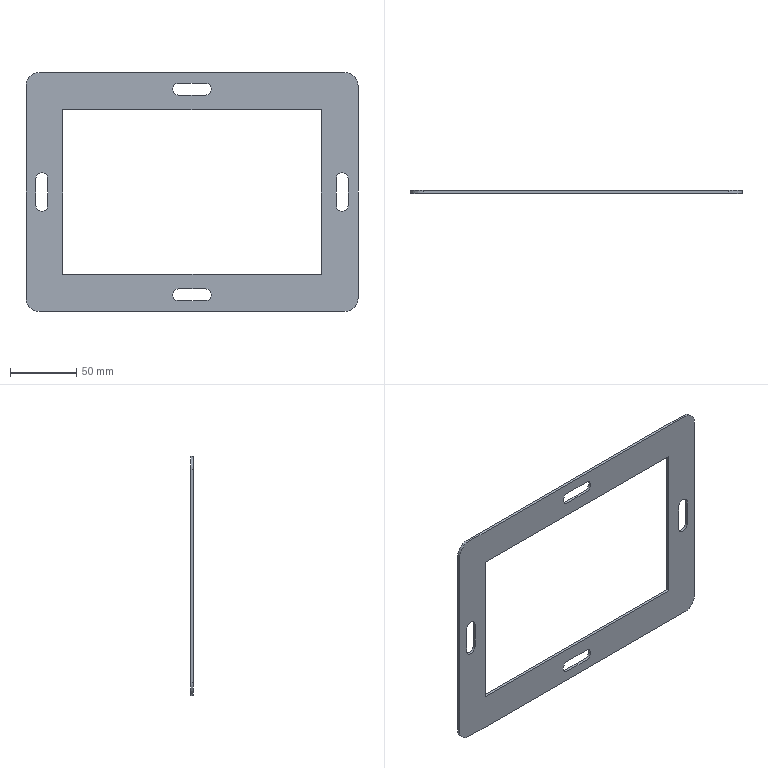Part | STEP file | JBJ-P-1003-01 | 1 solid | 30 faces | box 250 x 2 x 180 mm | volume 39519 mm3 | plane 18 | cylinder 12 | commonest cylinder face diameters 9 x8 20 x4
STEP:
#1=CARTESIAN_POINT('',(125.,2.,80.));
#2=VERTEX_POINT('',#1);
#3=CARTESIAN_POINT('',(125.,2.,-80.));
#4=VERTEX_POINT('',#3);
#5=CARTESIAN_POINT('',(125.,2.,-90.));
#6=DIRECTION('',(0.,0.,-1.));
#7=VECTOR('',#6,1000.);
#8=LINE('',#5,#7);
#9=EDGE_CURVE('',#2,#4,#8,.T.);
#10=ORIENTED_EDGE('',*,*,#9,.F.);
#11=CARTESIAN_POINT('',(125.,0.,80.));
#12=VERTEX_POINT('',#11);
#13=CARTESIAN_POINT('',(125.,2.,80.));
#14=DIRECTION('',(0.,-1.,0.));
#15=VECTOR('',#14,1000.);
#16=LINE('',#13,#15);
#17=EDGE_CURVE('',#2,#12,#16,.T.);
#18=ORIENTED_EDGE('',*,*,#17,.T.);
#19=CARTESIAN_POINT('',(125.,0.,-80.));
#20=VERTEX_POINT('',#19);
#21=CARTESIAN_POINT('',(125.,0.,-90.));
#22=DIRECTION('',(0.,0.,-1.));
#23=VECTOR('',#22,1000.);
#24=LINE('',#21,#23);
#25=EDGE_CURVE('',#12,#20,#24,.T.);
#26=ORIENTED_EDGE('',*,*,#25,.T.);
#27=CARTESIAN_POINT('',(125.,2.,-80.));
#28=DIRECTION('',(0.,1.,0.));
#29=VECTOR('',#28,1000.);
#30=LINE('',#27,#29);
#31=EDGE_CURVE('',#20,#4,#30,.T.);
#32=ORIENTED_EDGE('',*,*,#31,.T.);
#33=EDGE_LOOP('',(#10,#18,#26,#32));
#34=FACE_OUTER_BOUND('',#33,.T.);
#35=CARTESIAN_POINT('',(125.,2.,-90.));
#36=DIRECTION('',(-1.,0.,0.));
#37=DIRECTION('',(0.,0.,1.));
#38=AXIS2_PLACEMENT_3D('',#35,#36,#37);
#39=PLANE('',#38);
#40=ADVANCED_FACE('',(#34),#39,.F.);
#41=CARTESIAN_POINT('',(115.,2.,-90.));
#42=VERTEX_POINT('',#41);
#43=CARTESIAN_POINT('',(-115.,2.,-90.));
#44=VERTEX_POINT('',#43);
#45=CARTESIAN_POINT('',(-125.,2.,-90.));
#46=DIRECTION('',(-1.,0.,0.));
#47=VECTOR('',#46,1000.);
#48=LINE('',#45,#47);
#49=EDGE_CURVE('',#42,#44,#48,.T.);
#50=ORIENTED_EDGE('',*,*,#49,.F.);
#51=CARTESIAN_POINT('',(115.,0.,-90.));
#52=VERTEX_POINT('',#51);
#53=CARTESIAN_POINT('',(115.,2.,-90.));
#54=DIRECTION('',(0.,-1.,0.));
#55=VECTOR('',#54,1000.);
#56=LINE('',#53,#55);
#57=EDGE_CURVE('',#42,#52,#56,.T.);
#58=ORIENTED_EDGE('',*,*,#57,.T.);
#59=CARTESIAN_POINT('',(-115.,0.,-90.));
#60=VERTEX_POINT('',#59);
#61=CARTESIAN_POINT('',(-125.,0.,-90.));
#62=DIRECTION('',(-1.,0.,0.));
#63=VECTOR('',#62,1000.);
#64=LINE('',#61,#63);
#65=EDGE_CURVE('',#52,#60,#64,.T.);
#66=ORIENTED_EDGE('',*,*,#65,.T.);
#67=CARTESIAN_POINT('',(-115.,2.,-90.));
#68=DIRECTION('',(0.,1.,0.));
#69=VECTOR('',#68,1000.);
#70=LINE('',#67,#69);
#71=EDGE_CURVE('',#60,#44,#70,.T.);
#72=ORIENTED_EDGE('',*,*,#71,.T.);
#73=EDGE_LOOP('',(#50,#58,#66,#72));
#74=FACE_OUTER_BOUND('',#73,.T.);
#75=CARTESIAN_POINT('',(-125.,2.,-90.));
#76=DIRECTION('',(0.,0.,1.));
#77=DIRECTION('',(1.,0.,0.));
#78=AXIS2_PLACEMENT_3D('',#75,#76,#77);
#79=PLANE('',#78);
#80=ADVANCED_FACE('',(#74),#79,.F.);
#81=CARTESIAN_POINT('',(-125.,0.,-80.));
#82=VERTEX_POINT('',#81);
#83=CARTESIAN_POINT('',(-125.,0.,80.));
#84=VERTEX_POINT('',#83);
#85=CARTESIAN_POINT('',(-125.,0.,-90.));
#86=DIRECTION('',(0.,0.,1.));
#87=VECTOR('',#86,1000.);
#88=LINE('',#85,#87);
#89=EDGE_CURVE('',#82,#84,#88,.T.);
#90=ORIENTED_EDGE('',*,*,#89,.T.);
#91=CARTESIAN_POINT('',(-125.,2.,80.));
#92=VERTEX_POINT('',#91);
#93=CARTESIAN_POINT('',(-125.,2.,80.));
#94=DIRECTION('',(0.,1.,0.));
#95=VECTOR('',#94,1000.);
#96=LINE('',#93,#95);
#97=EDGE_CURVE('',#84,#92,#96,.T.);
#98=ORIENTED_EDGE('',*,*,#97,.T.);
#99=CARTESIAN_POINT('',(-125.,2.,-80.));
#100=VERTEX_POINT('',#99);
#101=CARTESIAN_POINT('',(-125.,2.,-90.));
#102=DIRECTION('',(0.,0.,1.));
#103=VECTOR('',#102,1000.);
#104=LINE('',#101,#103);
#105=EDGE_CURVE('',#100,#92,#104,.T.);
#106=ORIENTED_EDGE('',*,*,#105,.F.);
#107=CARTESIAN_POINT('',(-125.,2.,-80.));
#108=DIRECTION('',(0.,-1.,0.));
#109=VECTOR('',#108,1000.);
#110=LINE('',#107,#109);
#111=EDGE_CURVE('',#100,#82,#110,.T.);
#112=ORIENTED_EDGE('',*,*,#111,.T.);
#113=EDGE_LOOP('',(#90,#98,#106,#112));
#114=FACE_OUTER_BOUND('',#113,.T.);
#115=CARTESIAN_POINT('',(-125.,2.,-90.));
#116=DIRECTION('',(1.,0.,0.));
#117=DIRECTION('',(0.,0.,-1.));
#118=AXIS2_PLACEMENT_3D('',#115,#116,#117);
#119=PLANE('',#118);
#120=ADVANCED_FACE('',(#114),#119,.F.);
#121=CARTESIAN_POINT('',(-115.,2.,90.));
#122=VERTEX_POINT('',#121);
#123=CARTESIAN_POINT('',(115.,2.,90.));
#124=VERTEX_POINT('',#123);
#125=CARTESIAN_POINT('',(-125.,2.,90.));
#126=DIRECTION('',(1.,0.,0.));
#127=VECTOR('',#126,1000.);
#128=LINE('',#125,#127);
#129=EDGE_CURVE('',#122,#124,#128,.T.);
#130=ORIENTED_EDGE('',*,*,#129,.F.);
#131=CARTESIAN_POINT('',(-115.,0.,90.));
#132=VERTEX_POINT('',#131);
#133=CARTESIAN_POINT('',(-115.,2.,90.));
#134=DIRECTION('',(0.,-1.,0.));
#135=VECTOR('',#134,1000.);
#136=LINE('',#133,#135);
#137=EDGE_CURVE('',#122,#132,#136,.T.);
#138=ORIENTED_EDGE('',*,*,#137,.T.);
#139=CARTESIAN_POINT('',(115.,0.,90.));
#140=VERTEX_POINT('',#139);
#141=CARTESIAN_POINT('',(-125.,0.,90.));
#142=DIRECTION('',(1.,0.,0.));
#143=VECTOR('',#142,1000.);
#144=LINE('',#141,#143);
#145=EDGE_CURVE('',#132,#140,#144,.T.);
#146=ORIENTED_EDGE('',*,*,#145,.T.);
#147=CARTESIAN_POINT('',(115.,2.,90.));
#148=DIRECTION('',(0.,1.,0.));
#149=VECTOR('',#148,1000.);
#150=LINE('',#147,#149);
#151=EDGE_CURVE('',#140,#124,#150,.T.);
#152=ORIENTED_EDGE('',*,*,#151,.T.);
#153=EDGE_LOOP('',(#130,#138,#146,#152));
#154=FACE_OUTER_BOUND('',#153,.T.);
#155=CARTESIAN_POINT('',(-125.,2.,90.));
#156=DIRECTION('',(0.,0.,-1.));
#157=DIRECTION('',(-1.,0.,0.));
#158=AXIS2_PLACEMENT_3D('',#155,#156,#157);
#159=PLANE('',#158);
#160=ADVANCED_FACE('',(#154),#159,.F.);
#161=CARTESIAN_POINT('',(-108.5,2.,-10.));
#162=VERTEX_POINT('',#161);
#163=CARTESIAN_POINT('',(-117.5,2.,-10.));
#164=VERTEX_POINT('',#163);
#165=CARTESIAN_POINT('',(-113.,2.,-10.));
#166=DIRECTION('',(0.,1.,0.));
#167=DIRECTION('',(0.,0.,1.));
#168=AXIS2_PLACEMENT_3D('',#165,#166,#167);
#169=CIRCLE('',#168,4.5);
#170=EDGE_CURVE('',#162,#164,#169,.T.);
#171=ORIENTED_EDGE('',*,*,#170,.F.);
#172=CARTESIAN_POINT('',(-108.5,2.,10.));
#173=VERTEX_POINT('',#172);
#174=CARTESIAN_POINT('',(-108.5,2.,-10.));
#175=DIRECTION('',(0.,0.,-1.));
#176=VECTOR('',#175,1000.);
#177=LINE('',#174,#176);
#178=EDGE_CURVE('',#173,#162,#177,.T.);
#179=ORIENTED_EDGE('',*,*,#178,.F.);
#180=CARTESIAN_POINT('',(-117.5,2.,10.));
#181=VERTEX_POINT('',#180);
#182=CARTESIAN_POINT('',(-113.,2.,10.));
#183=DIRECTION('',(0.,1.,0.));
#184=DIRECTION('',(0.,0.,1.));
#185=AXIS2_PLACEMENT_3D('',#182,#183,#184);
#186=CIRCLE('',#185,4.5);
#187=EDGE_CURVE('',#181,#173,#186,.T.);
#188=ORIENTED_EDGE('',*,*,#187,.F.);
#189=CARTESIAN_POINT('',(-117.5,2.,-10.));
#190=DIRECTION('',(0.,0.,1.));
#191=VECTOR('',#190,1000.);
#192=LINE('',#189,#191);
#193=EDGE_CURVE('',#164,#181,#192,.T.);
#194=ORIENTED_EDGE('',*,*,#193,.F.);
#195=EDGE_LOOP('',(#171,#179,#188,#194));
#196=FACE_BOUND('',#195,.T.);
#197=CARTESIAN_POINT('',(117.5,2.,-10.));
#198=VERTEX_POINT('',#197);
#199=CARTESIAN_POINT('',(108.5,2.,-10.));
#200=VERTEX_POINT('',#199);
#201=CARTESIAN_POINT('',(113.,2.,-10.));
#202=DIRECTION('',(0.,1.,0.));
#203=DIRECTION('',(0.,0.,-1.));
#204=AXIS2_PLACEMENT_3D('',#201,#202,#203);
#205=CIRCLE('',#204,4.5);
#206=EDGE_CURVE('',#198,#200,#205,.T.);
#207=ORIENTED_EDGE('',*,*,#206,.F.);
#208=CARTESIAN_POINT('',(117.5,2.,10.));
#209=VERTEX_POINT('',#208);
#210=CARTESIAN_POINT('',(117.5,2.,-10.));
#211=DIRECTION('',(0.,0.,-1.));
#212=VECTOR('',#211,1000.);
#213=LINE('',#210,#212);
#214=EDGE_CURVE('',#209,#198,#213,.T.);
#215=ORIENTED_EDGE('',*,*,#214,.F.);
#216=CARTESIAN_POINT('',(108.5,2.,10.));
#217=VERTEX_POINT('',#216);
#218=CARTESIAN_POINT('',(113.,2.,10.));
#219=DIRECTION('',(0.,1.,0.));
#220=DIRECTION('',(0.,0.,-1.));
#221=AXIS2_PLACEMENT_3D('',#218,#219,#220);
#222=CIRCLE('',#221,4.5);
#223=EDGE_CURVE('',#217,#209,#222,.T.);
#224=ORIENTED_EDGE('',*,*,#223,.F.);
#225=CARTESIAN_POINT('',(108.5,2.,-10.));
#226=DIRECTION('',(0.,0.,1.));
#227=VECTOR('',#226,1000.);
#228=LINE('',#225,#227);
#229=EDGE_CURVE('',#200,#217,#228,.T.);
#230=ORIENTED_EDGE('',*,*,#229,.F.);
#231=EDGE_LOOP('',(#207,#215,#224,#230));
#232=FACE_BOUND('',#231,.T.);
#233=CARTESIAN_POINT('',(-10.,2.,73.));
#234=VERTEX_POINT('',#233);
#235=CARTESIAN_POINT('',(-10.,2.,82.));
#236=VERTEX_POINT('',#235);
#237=CARTESIAN_POINT('',(-10.,2.,77.5));
#238=DIRECTION('',(0.,1.,0.));
#239=DIRECTION('',(0.,0.,-1.));
#240=AXIS2_PLACEMENT_3D('',#237,#238,#239);
#241=CIRCLE('',#240,4.5);
#242=EDGE_CURVE('',#234,#236,#241,.T.);
#243=ORIENTED_EDGE('',*,*,#242,.F.);
#244=CARTESIAN_POINT('',(10.,2.,73.));
#245=VERTEX_POINT('',#244);
#246=CARTESIAN_POINT('',(-10.,2.,73.));
#247=DIRECTION('',(-1.,0.,0.));
#248=VECTOR('',#247,1000.);
#249=LINE('',#246,#248);
#250=EDGE_CURVE('',#245,#234,#249,.T.);
#251=ORIENTED_EDGE('',*,*,#250,.F.);
#252=CARTESIAN_POINT('',(10.,2.,82.));
#253=VERTEX_POINT('',#252);
#254=CARTESIAN_POINT('',(10.,2.,77.5));
#255=DIRECTION('',(0.,1.,0.));
#256=DIRECTION('',(0.,0.,-1.));
#257=AXIS2_PLACEMENT_3D('',#254,#255,#256);
#258=CIRCLE('',#257,4.5);
#259=EDGE_CURVE('',#253,#245,#258,.T.);
#260=ORIENTED_EDGE('',*,*,#259,.F.);
#261=CARTESIAN_POINT('',(-10.,2.,82.));
#262=DIRECTION('',(1.,0.,0.));
#263=VECTOR('',#262,1000.);
#264=LINE('',#261,#263);
#265=EDGE_CURVE('',#236,#253,#264,.T.);
#266=ORIENTED_EDGE('',*,*,#265,.F.);
#267=EDGE_LOOP('',(#243,#251,#260,#266));
#268=FACE_BOUND('',#267,.T.);
#269=CARTESIAN_POINT('',(97.5,2.,62.));
#270=VERTEX_POINT('',#269);
#271=CARTESIAN_POINT('',(97.5,2.,-62.));
#272=VERTEX_POINT('',#271);
#273=CARTESIAN_POINT('',(97.5,2.,-62.));
#274=DIRECTION('',(0.,0.,-1.));
#275=VECTOR('',#274,1000.);
#276=LINE('',#273,#275);
#277=EDGE_CURVE('',#270,#272,#276,.T.);
#278=ORIENTED_EDGE('',*,*,#277,.F.);
#279=CARTESIAN_POINT('',(-97.5,2.,62.));
#280=VERTEX_POINT('',#279);
#281=CARTESIAN_POINT('',(-97.5,2.,62.));
#282=DIRECTION('',(1.,0.,0.));
#283=VECTOR('',#282,1000.);
#284=LINE('',#281,#283);
#285=EDGE_CURVE('',#280,#270,#284,.T.);
#286=ORIENTED_EDGE('',*,*,#285,.F.);
#287=CARTESIAN_POINT('',(-97.5,2.,-62.));
#288=VERTEX_POINT('',#287);
#289=CARTESIAN_POINT('',(-97.5,2.,-62.));
#290=DIRECTION('',(0.,0.,1.));
#291=VECTOR('',#290,1000.);
#292=LINE('',#289,#291);
#293=EDGE_CURVE('',#288,#280,#292,.T.);
#294=ORIENTED_EDGE('',*,*,#293,.F.);
#295=CARTESIAN_POINT('',(-97.5,2.,-62.));
#296=DIRECTION('',(-1.,0.,0.));
#297=VECTOR('',#296,1000.);
#298=LINE('',#295,#297);
#299=EDGE_CURVE('',#272,#288,#298,.T.);
#300=ORIENTED_EDGE('',*,*,#299,.F.);
#301=EDGE_LOOP('',(#278,#286,#294,#300));
#302=FACE_BOUND('',#301,.T.);
#303=CARTESIAN_POINT('',(-10.,2.,-82.));
#304=VERTEX_POINT('',#303);
#305=CARTESIAN_POINT('',(-10.,2.,-73.));
#306=VERTEX_POINT('',#305);
#307=CARTESIAN_POINT('',(-10.,2.,-77.5));
#308=DIRECTION('',(0.,1.,0.));
#309=DIRECTION('',(0.,0.,1.));
#310=AXIS2_PLACEMENT_3D('',#307,#308,#309);
#311=CIRCLE('',#310,4.5);
#312=EDGE_CURVE('',#304,#306,#311,.T.);
#313=ORIENTED_EDGE('',*,*,#312,.F.);
#314=CARTESIAN_POINT('',(10.,2.,-82.));
#315=VERTEX_POINT('',#314);
#316=CARTESIAN_POINT('',(-10.,2.,-82.));
#317=DIRECTION('',(-1.,0.,0.));
#318=VECTOR('',#317,1000.);
#319=LINE('',#316,#318);
#320=EDGE_CURVE('',#315,#304,#319,.T.);
#321=ORIENTED_EDGE('',*,*,#320,.F.);
#322=CARTESIAN_POINT('',(10.,2.,-73.));
#323=VERTEX_POINT('',#322);
#324=CARTESIAN_POINT('',(10.,2.,-77.5));
#325=DIRECTION('',(0.,1.,0.));
#326=DIRECTION('',(0.,0.,1.));
#327=AXIS2_PLACEMENT_3D('',#324,#325,#326);
#328=CIRCLE('',#327,4.5);
#329=EDGE_CURVE('',#323,#315,#328,.T.);
#330=ORIENTED_EDGE('',*,*,#329,.F.);
#331=CARTESIAN_POINT('',(-10.,2.,-73.));
#332=DIRECTION('',(1.,0.,0.));
#333=VECTOR('',#332,1000.);
#334=LINE('',#331,#333);
#335=EDGE_CURVE('',#306,#323,#334,.T.);
#336=ORIENTED_EDGE('',*,*,#335,.F.);
#337=EDGE_LOOP('',(#313,#321,#330,#336));
#338=FACE_BOUND('',#337,.T.);
#339=ORIENTED_EDGE('',*,*,#105,.T.);
#340=CARTESIAN_POINT('',(-115.,2.,80.));
#341=DIRECTION('',(0.,1.,0.));
#342=DIRECTION('',(0.,0.,1.));
#343=AXIS2_PLACEMENT_3D('',#340,#341,#342);
#344=CIRCLE('',#343,10.);
#345=EDGE_CURVE('',#92,#122,#344,.T.);
#346=ORIENTED_EDGE('',*,*,#345,.T.);
#347=ORIENTED_EDGE('',*,*,#129,.T.);
#348=CARTESIAN_POINT('',(115.,2.,80.));
#349=DIRECTION('',(0.,1.,0.));
#350=DIRECTION('',(0.,0.,1.));
#351=AXIS2_PLACEMENT_3D('',#348,#349,#350);
#352=CIRCLE('',#351,10.);
#353=EDGE_CURVE('',#124,#2,#352,.T.);
#354=ORIENTED_EDGE('',*,*,#353,.T.);
#355=ORIENTED_EDGE('',*,*,#9,.T.);
#356=CARTESIAN_POINT('',(115.,2.,-80.));
#357=DIRECTION('',(0.,1.,0.));
#358=DIRECTION('',(0.,0.,1.));
#359=AXIS2_PLACEMENT_3D('',#356,#357,#358);
#360=CIRCLE('',#359,10.);
#361=EDGE_CURVE('',#4,#42,#360,.T.);
#362=ORIENTED_EDGE('',*,*,#361,.T.);
#363=ORIENTED_EDGE('',*,*,#49,.T.);
#364=CARTESIAN_POINT('',(-115.,2.,-80.));
#365=DIRECTION('',(0.,1.,0.));
#366=DIRECTION('',(0.,0.,1.));
#367=AXIS2_PLACEMENT_3D('',#364,#365,#366);
#368=CIRCLE('',#367,10.);
#369=EDGE_CURVE('',#44,#100,#368,.T.);
#370=ORIENTED_EDGE('',*,*,#369,.T.);
#371=EDGE_LOOP('',(#339,#346,#347,#354,#355,#362,#363,#370));
#372=FACE_OUTER_BOUND('',#371,.T.);
#373=CARTESIAN_POINT('',(0.,2.,0.));
#374=DIRECTION('',(0.,1.,0.));
#375=DIRECTION('',(0.,0.,1.));
#376=AXIS2_PLACEMENT_3D('',#373,#374,#375);
#377=PLANE('',#376);
#378=ADVANCED_FACE('',(#196,#232,#268,#302,#338,#372),#377,.T.);
#379=CARTESIAN_POINT('',(-108.5,0.,10.));
#380=VERTEX_POINT('',#379);
#381=CARTESIAN_POINT('',(-108.5,0.,-10.));
#382=VERTEX_POINT('',#381);
#383=CARTESIAN_POINT('',(-108.5,0.,-10.));
#384=DIRECTION('',(0.,0.,-1.));
#385=VECTOR('',#384,1000.);
#386=LINE('',#383,#385);
#387=EDGE_CURVE('',#380,#382,#386,.T.);
#388=ORIENTED_EDGE('',*,*,#387,.T.);
#389=CARTESIAN_POINT('',(-117.5,0.,-10.));
#390=VERTEX_POINT('',#389);
#391=CARTESIAN_POINT('',(-113.,0.,-10.));
#392=DIRECTION('',(0.,1.,0.));
#393=DIRECTION('',(0.,0.,1.));
#394=AXIS2_PLACEMENT_3D('',#391,#392,#393);
#395=CIRCLE('',#394,4.5);
#396=EDGE_CURVE('',#382,#390,#395,.T.);
#397=ORIENTED_EDGE('',*,*,#396,.T.);
#398=CARTESIAN_POINT('',(-117.5,0.,10.));
#399=VERTEX_POINT('',#398);
#400=CARTESIAN_POINT('',(-117.5,0.,-10.));
#401=DIRECTION('',(0.,0.,1.));
#402=VECTOR('',#401,1000.);
#403=LINE('',#400,#402);
#404=EDGE_CURVE('',#390,#399,#403,.T.);
#405=ORIENTED_EDGE('',*,*,#404,.T.);
#406=CARTESIAN_POINT('',(-113.,0.,10.));
#407=DIRECTION('',(0.,1.,0.));
#408=DIRECTION('',(0.,0.,1.));
#409=AXIS2_PLACEMENT_3D('',#406,#407,#408);
#410=CIRCLE('',#409,4.5);
#411=EDGE_CURVE('',#399,#380,#410,.T.);
#412=ORIENTED_EDGE('',*,*,#411,.T.);
#413=EDGE_LOOP('',(#388,#397,#405,#412));
#414=FACE_BOUND('',#413,.T.);
#415=CARTESIAN_POINT('',(117.5,0.,10.));
#416=VERTEX_POINT('',#415);
#417=CARTESIAN_POINT('',(117.5,0.,-10.));
#418=VERTEX_POINT('',#417);
#419=CARTESIAN_POINT('',(117.5,0.,-10.));
#420=DIRECTION('',(0.,0.,-1.));
#421=VECTOR('',#420,1000.);
#422=LINE('',#419,#421);
#423=EDGE_CURVE('',#416,#418,#422,.T.);
#424=ORIENTED_EDGE('',*,*,#423,.T.);
#425=CARTESIAN_POINT('',(108.5,0.,-10.));
#426=VERTEX_POINT('',#425);
#427=CARTESIAN_POINT('',(113.,0.,-10.));
#428=DIRECTION('',(0.,1.,0.));
#429=DIRECTION('',(0.,0.,-1.));
#430=AXIS2_PLACEMENT_3D('',#427,#428,#429);
#431=CIRCLE('',#430,4.5);
#432=EDGE_CURVE('',#418,#426,#431,.T.);
#433=ORIENTED_EDGE('',*,*,#432,.T.);
#434=CARTESIAN_POINT('',(108.5,0.,10.));
#435=VERTEX_POINT('',#434);
#436=CARTESIAN_POINT('',(108.5,0.,-10.));
#437=DIRECTION('',(0.,0.,1.));
#438=VECTOR('',#437,1000.);
#439=LINE('',#436,#438);
#440=EDGE_CURVE('',#426,#435,#439,.T.);
#441=ORIENTED_EDGE('',*,*,#440,.T.);
#442=CARTESIAN_POINT('',(113.,0.,10.));
#443=DIRECTION('',(0.,1.,0.));
#444=DIRECTION('',(0.,0.,-1.));
#445=AXIS2_PLACEMENT_3D('',#442,#443,#444);
#446=CIRCLE('',#445,4.5);
#447=EDGE_CURVE('',#435,#416,#446,.T.);
#448=ORIENTED_EDGE('',*,*,#447,.T.);
#449=EDGE_LOOP('',(#424,#433,#441,#448));
#450=FACE_BOUND('',#449,.T.);
#451=CARTESIAN_POINT('',(10.,0.,73.));
#452=VERTEX_POINT('',#451);
#453=CARTESIAN_POINT('',(-10.,0.,73.));
#454=VERTEX_POINT('',#453);
#455=CARTESIAN_POINT('',(-10.,0.,73.));
#456=DIRECTION('',(-1.,0.,0.));
#457=VECTOR('',#456,1000.);
#458=LINE('',#455,#457);
#459=EDGE_CURVE('',#452,#454,#458,.T.);
#460=ORIENTED_EDGE('',*,*,#459,.T.);
#461=CARTESIAN_POINT('',(-10.,0.,82.));
#462=VERTEX_POINT('',#461);
#463=CARTESIAN_POINT('',(-10.,0.,77.5));
#464=DIRECTION('',(0.,1.,0.));
#465=DIRECTION('',(0.,0.,-1.));
#466=AXIS2_PLACEMENT_3D('',#463,#464,#465);
#467=CIRCLE('',#466,4.5);
#468=EDGE_CURVE('',#454,#462,#467,.T.);
#469=ORIENTED_EDGE('',*,*,#468,.T.);
#470=CARTESIAN_POINT('',(10.,0.,82.));
#471=VERTEX_POINT('',#470);
#472=CARTESIAN_POINT('',(-10.,0.,82.));
#473=DIRECTION('',(1.,0.,0.));
#474=VECTOR('',#473,1000.);
#475=LINE('',#472,#474);
#476=EDGE_CURVE('',#462,#471,#475,.T.);
#477=ORIENTED_EDGE('',*,*,#476,.T.);
#478=CARTESIAN_POINT('',(10.,0.,77.5));
#479=DIRECTION('',(0.,1.,0.));
#480=DIRECTION('',(0.,0.,-1.));
#481=AXIS2_PLACEMENT_3D('',#478,#479,#480);
#482=CIRCLE('',#481,4.5);
#483=EDGE_CURVE('',#471,#452,#482,.T.);
#484=ORIENTED_EDGE('',*,*,#483,.T.);
#485=EDGE_LOOP('',(#460,#469,#477,#484));
#486=FACE_BOUND('',#485,.T.);
#487=CARTESIAN_POINT('',(-97.5,0.,62.));
#488=VERTEX_POINT('',#487);
#489=CARTESIAN_POINT('',(97.5,0.,62.));
#490=VERTEX_POINT('',#489);
#491=CARTESIAN_POINT('',(-97.5,0.,62.));
#492=DIRECTION('',(1.,0.,0.));
#493=VECTOR('',#492,1000.);
#494=LINE('',#491,#493);
#495=EDGE_CURVE('',#488,#490,#494,.T.);
#496=ORIENTED_EDGE('',*,*,#495,.T.);
#497=CARTESIAN_POINT('',(97.5,0.,-62.));
#498=VERTEX_POINT('',#497);
#499=CARTESIAN_POINT('',(97.5,0.,-62.));
#500=DIRECTION('',(0.,0.,-1.));
#501=VECTOR('',#500,1000.);
#502=LINE('',#499,#501);
#503=EDGE_CURVE('',#490,#498,#502,.T.);
#504=ORIENTED_EDGE('',*,*,#503,.T.);
#505=CARTESIAN_POINT('',(-97.5,0.,-62.));
#506=VERTEX_POINT('',#505);
#507=CARTESIAN_POINT('',(-97.5,0.,-62.));
#508=DIRECTION('',(-1.,0.,0.));
#509=VECTOR('',#508,1000.);
#510=LINE('',#507,#509);
#511=EDGE_CURVE('',#498,#506,#510,.T.);
#512=ORIENTED_EDGE('',*,*,#511,.T.);
#513=CARTESIAN_POINT('',(-97.5,0.,-62.));
#514=DIRECTION('',(0.,0.,1.));
#515=VECTOR('',#514,1000.);
#516=LINE('',#513,#515);
#517=EDGE_CURVE('',#506,#488,#516,.T.);
#518=ORIENTED_EDGE('',*,*,#517,.T.);
#519=EDGE_LOOP('',(#496,#504,#512,#518));
#520=FACE_BOUND('',#519,.T.);
#521=CARTESIAN_POINT('',(10.,0.,-82.));
#522=VERTEX_POINT('',#521);
#523=CARTESIAN_POINT('',(-10.,0.,-82.));
#524=VERTEX_POINT('',#523);
#525=CARTESIAN_POINT('',(-10.,0.,-82.));
#526=DIRECTION('',(-1.,0.,0.));
#527=VECTOR('',#526,1000.);
#528=LINE('',#525,#527);
#529=EDGE_CURVE('',#522,#524,#528,.T.);
#530=ORIENTED_EDGE('',*,*,#529,.T.);
#531=CARTESIAN_POINT('',(-10.,0.,-73.));
#532=VERTEX_POINT('',#531);
#533=CARTESIAN_POINT('',(-10.,0.,-77.5));
#534=DIRECTION('',(0.,1.,0.));
#535=DIRECTION('',(0.,0.,1.));
#536=AXIS2_PLACEMENT_3D('',#533,#534,#535);
#537=CIRCLE('',#536,4.5);
#538=EDGE_CURVE('',#524,#532,#537,.T.);
#539=ORIENTED_EDGE('',*,*,#538,.T.);
#540=CARTESIAN_POINT('',(10.,0.,-73.));
#541=VERTEX_POINT('',#540);
#542=CARTESIAN_POINT('',(-10.,0.,-73.));
#543=DIRECTION('',(1.,0.,0.));
#544=VECTOR('',#543,1000.);
#545=LINE('',#542,#544);
#546=EDGE_CURVE('',#532,#541,#545,.T.);
#547=ORIENTED_EDGE('',*,*,#546,.T.);
#548=CARTESIAN_POINT('',(10.,0.,-77.5));
#549=DIRECTION('',(0.,1.,0.));
#550=DIRECTION('',(0.,0.,1.));
#551=AXIS2_PLACEMENT_3D('',#548,#549,#550);
#552=CIRCLE('',#551,4.5);
#553=EDGE_CURVE('',#541,#522,#552,.T.);
#554=ORIENTED_EDGE('',*,*,#553,.T.);
#555=EDGE_LOOP('',(#530,#539,#547,#554));
#556=FACE_BOUND('',#555,.T.);
#557=ORIENTED_EDGE('',*,*,#145,.F.);
#558=CARTESIAN_POINT('',(-115.,0.,80.));
#559=DIRECTION('',(0.,-1.,0.));
#560=DIRECTION('',(0.,0.,1.));
#561=AXIS2_PLACEMENT_3D('',#558,#559,#560);
#562=CIRCLE('',#561,10.);
#563=EDGE_CURVE('',#132,#84,#562,.T.);
#564=ORIENTED_EDGE('',*,*,#563,.T.);
#565=ORIENTED_EDGE('',*,*,#89,.F.);
#566=CARTESIAN_POINT('',(-115.,0.,-80.));
#567=DIRECTION('',(0.,-1.,0.));
#568=DIRECTION('',(0.,0.,1.));
#569=AXIS2_PLACEMENT_3D('',#566,#567,#568);
#570=CIRCLE('',#569,10.);
#571=EDGE_CURVE('',#82,#60,#570,.T.);
#572=ORIENTED_EDGE('',*,*,#571,.T.);
#573=ORIENTED_EDGE('',*,*,#65,.F.);
#574=CARTESIAN_POINT('',(115.,0.,-80.));
#575=DIRECTION('',(0.,-1.,0.));
#576=DIRECTION('',(0.,0.,1.));
#577=AXIS2_PLACEMENT_3D('',#574,#575,#576);
#578=CIRCLE('',#577,10.);
#579=EDGE_CURVE('',#52,#20,#578,.T.);
#580=ORIENTED_EDGE('',*,*,#579,.T.);
#581=ORIENTED_EDGE('',*,*,#25,.F.);
#582=CARTESIAN_POINT('',(115.,0.,80.));
#583=DIRECTION('',(0.,-1.,0.));
#584=DIRECTION('',(0.,0.,1.));
#585=AXIS2_PLACEMENT_3D('',#582,#583,#584);
#586=CIRCLE('',#585,10.);
#587=EDGE_CURVE('',#12,#140,#586,.T.);
#588=ORIENTED_EDGE('',*,*,#587,.T.);
#589=EDGE_LOOP('',(#557,#564,#565,#572,#573,#580,#581,#588));
#590=FACE_OUTER_BOUND('',#589,.T.);
#591=CARTESIAN_POINT('',(0.,0.,0.));
#592=DIRECTION('',(0.,1.,0.));
#593=DIRECTION('',(0.,0.,1.));
#594=AXIS2_PLACEMENT_3D('',#591,#592,#593);
#595=PLANE('',#594);
#596=ADVANCED_FACE('',(#414,#450,#486,#520,#556,#590),#595,.F.);
#597=ORIENTED_EDGE('',*,*,#312,.T.);
#598=CARTESIAN_POINT('',(-10.,0.,-73.));
#599=DIRECTION('',(0.,1.,0.));
#600=VECTOR('',#599,1000.);
#601=LINE('',#598,#600);
#602=EDGE_CURVE('',#532,#306,#601,.T.);
#603=ORIENTED_EDGE('',*,*,#602,.F.);
#604=ORIENTED_EDGE('',*,*,#538,.F.);
#605=CARTESIAN_POINT('',(-10.,0.,-82.));
#606=DIRECTION('',(0.,1.,0.));
#607=VECTOR('',#606,1000.);
#608=LINE('',#605,#607);
#609=EDGE_CURVE('',#524,#304,#608,.T.);
#610=ORIENTED_EDGE('',*,*,#609,.T.);
#611=EDGE_LOOP('',(#597,#603,#604,#610));
#612=FACE_OUTER_BOUND('',#611,.T.);
#613=CARTESIAN_POINT('',(-10.,0.,-77.5));
#614=DIRECTION('',(0.,1.,0.));
#615=DIRECTION('',(0.,0.,1.));
#616=AXIS2_PLACEMENT_3D('',#613,#614,#615);
#617=CYLINDRICAL_SURFACE('',#616,4.5);
#618=ADVANCED_FACE('',(#612),#617,.F.);
#619=ORIENTED_EDGE('',*,*,#320,.T.);
#620=ORIENTED_EDGE('',*,*,#609,.F.);
#621=ORIENTED_EDGE('',*,*,#529,.F.);
#622=CARTESIAN_POINT('',(10.,0.,-82.));
#623=DIRECTION('',(0.,1.,0.));
#624=VECTOR('',#623,1000.);
#625=LINE('',#622,#624);
#626=EDGE_CURVE('',#522,#315,#625,.T.);
#627=ORIENTED_EDGE('',*,*,#626,.T.);
#628=EDGE_LOOP('',(#619,#620,#621,#627));
#629=FACE_OUTER_BOUND('',#628,.T.);
#630=CARTESIAN_POINT('',(-10.,0.,-82.));
#631=DIRECTION('',(0.,0.,-1.));
#632=DIRECTION('',(-1.,0.,0.));
#633=AXIS2_PLACEMENT_3D('',#630,#631,#632);
#634=PLANE('',#633);
#635=ADVANCED_FACE('',(#629),#634,.F.);
#636=ORIENTED_EDGE('',*,*,#329,.T.);
#637=ORIENTED_EDGE('',*,*,#626,.F.);
#638=ORIENTED_EDGE('',*,*,#553,.F.);
#639=CARTESIAN_POINT('',(10.,0.,-73.));
#640=DIRECTION('',(0.,1.,0.));
#641=VECTOR('',#640,1000.);
#642=LINE('',#639,#641);
#643=EDGE_CURVE('',#541,#323,#642,.T.);
#644=ORIENTED_EDGE('',*,*,#643,.T.);
#645=EDGE_LOOP('',(#636,#637,#638,#644));
#646=FACE_OUTER_BOUND('',#645,.T.);
#647=CARTESIAN_POINT('',(10.,0.,-77.5));
#648=DIRECTION('',(0.,1.,0.));
#649=DIRECTION('',(0.,0.,1.));
#650=AXIS2_PLACEMENT_3D('',#647,#648,#649);
#651=CYLINDRICAL_SURFACE('',#650,4.5);
#652=ADVANCED_FACE('',(#646),#651,.F.);
#653=ORIENTED_EDGE('',*,*,#335,.T.);
#654=ORIENTED_EDGE('',*,*,#643,.F.);
#655=ORIENTED_EDGE('',*,*,#546,.F.);
#656=ORIENTED_EDGE('',*,*,#602,.T.);
#657=EDGE_LOOP('',(#653,#654,#655,#656));
#658=FACE_OUTER_BOUND('',#657,.T.);
#659=CARTESIAN_POINT('',(-10.,0.,-73.));
#660=DIRECTION('',(0.,0.,1.));
#661=DIRECTION('',(1.,0.,0.));
#662=AXIS2_PLACEMENT_3D('',#659,#660,#661);
#663=PLANE('',#662);
#664=ADVANCED_FACE('',(#658),#663,.F.);
#665=ORIENTED_EDGE('',*,*,#277,.T.);
#666=CARTESIAN_POINT('',(97.5,0.,-62.));
#667=DIRECTION('',(0.,1.,0.));
#668=VECTOR('',#667,1000.);
#669=LINE('',#666,#668);
#670=EDGE_CURVE('',#498,#272,#669,.T.);
#671=ORIENTED_EDGE('',*,*,#670,.F.);
#672=ORIENTED_EDGE('',*,*,#503,.F.);
#673=CARTESIAN_POINT('',(97.5,0.,62.));
#674=DIRECTION('',(0.,1.,0.));
#675=VECTOR('',#674,1000.);
#676=LINE('',#673,#675);
#677=EDGE_CURVE('',#490,#270,#676,.T.);
#678=ORIENTED_EDGE('',*,*,#677,.T.);
#679=EDGE_LOOP('',(#665,#671,#672,#678));
#680=FACE_OUTER_BOUND('',#679,.T.);
#681=CARTESIAN_POINT('',(97.5,0.,-62.));
#682=DIRECTION('',(1.,0.,0.));
#683=DIRECTION('',(0.,0.,-1.));
#684=AXIS2_PLACEMENT_3D('',#681,#682,#683);
#685=PLANE('',#684);
#686=ADVANCED_FACE('',(#680),#685,.F.);
#687=ORIENTED_EDGE('',*,*,#285,.T.);
#688=ORIENTED_EDGE('',*,*,#677,.F.);
#689=ORIENTED_EDGE('',*,*,#495,.F.);
#690=CARTESIAN_POINT('',(-97.5,0.,62.));
#691=DIRECTION('',(0.,1.,0.));
#692=VECTOR('',#691,1000.);
#693=LINE('',#690,#692);
#694=EDGE_CURVE('',#488,#280,#693,.T.);
#695=ORIENTED_EDGE('',*,*,#694,.T.);
#696=EDGE_LOOP('',(#687,#688,#689,#695));
#697=FACE_OUTER_BOUND('',#696,.T.);
#698=CARTESIAN_POINT('',(-97.5,0.,62.));
#699=DIRECTION('',(0.,0.,1.));
#700=DIRECTION('',(1.,0.,0.));
#701=AXIS2_PLACEMENT_3D('',#698,#699,#700);
#702=PLANE('',#701);
#703=ADVANCED_FACE('',(#697),#702,.F.);
#704=ORIENTED_EDGE('',*,*,#293,.T.);
#705=ORIENTED_EDGE('',*,*,#694,.F.);
#706=ORIENTED_EDGE('',*,*,#517,.F.);
#707=CARTESIAN_POINT('',(-97.5,0.,-62.));
#708=DIRECTION('',(0.,1.,0.));
#709=VECTOR('',#708,1000.);
#710=LINE('',#707,#709);
#711=EDGE_CURVE('',#506,#288,#710,.T.);
#712=ORIENTED_EDGE('',*,*,#711,.T.);
#713=EDGE_LOOP('',(#704,#705,#706,#712));
#714=FACE_OUTER_BOUND('',#713,.T.);
#715=CARTESIAN_POINT('',(-97.5,0.,-62.));
#716=DIRECTION('',(-1.,0.,0.));
#717=DIRECTION('',(0.,0.,1.));
#718=AXIS2_PLACEMENT_3D('',#715,#716,#717);
#719=PLANE('',#718);
#720=ADVANCED_FACE('',(#714),#719,.F.);
#721=ORIENTED_EDGE('',*,*,#299,.T.);
#722=ORIENTED_EDGE('',*,*,#711,.F.);
#723=ORIENTED_EDGE('',*,*,#511,.F.);
#724=ORIENTED_EDGE('',*,*,#670,.T.);
#725=EDGE_LOOP('',(#721,#722,#723,#724));
#726=FACE_OUTER_BOUND('',#725,.T.);
#727=CARTESIAN_POINT('',(-97.5,0.,-62.));
#728=DIRECTION('',(0.,0.,-1.));
#729=DIRECTION('',(-1.,0.,0.));
#730=AXIS2_PLACEMENT_3D('',#727,#728,#729);
#731=PLANE('',#730);
#732=ADVANCED_FACE('',(#726),#731,.F.);
#733=ORIENTED_EDGE('',*,*,#242,.T.);
#734=CARTESIAN_POINT('',(-10.,0.,82.));
#735=DIRECTION('',(0.,1.,0.));
#736=VECTOR('',#735,1000.);
#737=LINE('',#734,#736);
#738=EDGE_CURVE('',#462,#236,#737,.T.);
#739=ORIENTED_EDGE('',*,*,#738,.F.);
#740=ORIENTED_EDGE('',*,*,#468,.F.);
#741=CARTESIAN_POINT('',(-10.,0.,73.));
#742=DIRECTION('',(0.,1.,0.));
#743=VECTOR('',#742,1000.);
#744=LINE('',#741,#743);
#745=EDGE_CURVE('',#454,#234,#744,.T.);
#746=ORIENTED_EDGE('',*,*,#745,.T.);
#747=EDGE_LOOP('',(#733,#739,#740,#746));
#748=FACE_OUTER_BOUND('',#747,.T.);
#749=CARTESIAN_POINT('',(-10.,0.,77.5));
#750=DIRECTION('',(0.,1.,0.));
#751=DIRECTION('',(0.,0.,1.));
#752=AXIS2_PLACEMENT_3D('',#749,#750,#751);
#753=CYLINDRICAL_SURFACE('',#752,4.5);
#754=ADVANCED_FACE('',(#748),#753,.F.);
#755=ORIENTED_EDGE('',*,*,#250,.T.);
#756=ORIENTED_EDGE('',*,*,#745,.F.);
#757=ORIENTED_EDGE('',*,*,#459,.F.);
#758=CARTESIAN_POINT('',(10.,0.,73.));
#759=DIRECTION('',(0.,1.,0.));
#760=VECTOR('',#759,1000.);
#761=LINE('',#758,#760);
#762=EDGE_CURVE('',#452,#245,#761,.T.);
#763=ORIENTED_EDGE('',*,*,#762,.T.);
#764=EDGE_LOOP('',(#755,#756,#757,#763));
#765=FACE_OUTER_BOUND('',#764,.T.);
#766=CARTESIAN_POINT('',(-10.,0.,73.));
#767=DIRECTION('',(0.,0.,-1.));
#768=DIRECTION('',(-1.,0.,0.));
#769=AXIS2_PLACEMENT_3D('',#766,#767,#768);
#770=PLANE('',#769);
#771=ADVANCED_FACE('',(#765),#770,.F.);
#772=ORIENTED_EDGE('',*,*,#259,.T.);
#773=ORIENTED_EDGE('',*,*,#762,.F.);
#774=ORIENTED_EDGE('',*,*,#483,.F.);
#775=CARTESIAN_POINT('',(10.,0.,82.));
#776=DIRECTION('',(0.,1.,0.));
#777=VECTOR('',#776,1000.);
#778=LINE('',#775,#777);
#779=EDGE_CURVE('',#471,#253,#778,.T.);
#780=ORIENTED_EDGE('',*,*,#779,.T.);
#781=EDGE_LOOP('',(#772,#773,#774,#780));
#782=FACE_OUTER_BOUND('',#781,.T.);
#783=CARTESIAN_POINT('',(10.,0.,77.5));
#784=DIRECTION('',(0.,1.,0.));
#785=DIRECTION('',(0.,0.,1.));
#786=AXIS2_PLACEMENT_3D('',#783,#784,#785);
#787=CYLINDRICAL_SURFACE('',#786,4.5);
#788=ADVANCED_FACE('',(#782),#787,.F.);
#789=ORIENTED_EDGE('',*,*,#265,.T.);
#790=ORIENTED_EDGE('',*,*,#779,.F.);
#791=ORIENTED_EDGE('',*,*,#476,.F.);
#792=ORIENTED_EDGE('',*,*,#738,.T.);
#793=EDGE_LOOP('',(#789,#790,#791,#792));
#794=FACE_OUTER_BOUND('',#793,.T.);
#795=CARTESIAN_POINT('',(-10.,0.,82.));
#796=DIRECTION('',(0.,0.,1.));
#797=DIRECTION('',(1.,0.,0.));
#798=AXIS2_PLACEMENT_3D('',#795,#796,#797);
#799=PLANE('',#798);
#800=ADVANCED_FACE('',(#794),#799,.F.);
#801=ORIENTED_EDGE('',*,*,#206,.T.);
#802=CARTESIAN_POINT('',(108.5,0.,-10.));
#803=DIRECTION('',(0.,1.,0.));
#804=VECTOR('',#803,1000.);
#805=LINE('',#802,#804);
#806=EDGE_CURVE('',#426,#200,#805,.T.);
#807=ORIENTED_EDGE('',*,*,#806,.F.);
#808=ORIENTED_EDGE('',*,*,#432,.F.);
#809=CARTESIAN_POINT('',(117.5,0.,-10.));
#810=DIRECTION('',(0.,1.,0.));
#811=VECTOR('',#810,1000.);
#812=LINE('',#809,#811);
#813=EDGE_CURVE('',#418,#198,#812,.T.);
#814=ORIENTED_EDGE('',*,*,#813,.T.);
#815=EDGE_LOOP('',(#801,#807,#808,#814));
#816=FACE_OUTER_BOUND('',#815,.T.);
#817=CARTESIAN_POINT('',(113.,0.,-10.));
#818=DIRECTION('',(0.,1.,0.));
#819=DIRECTION('',(0.,0.,1.));
#820=AXIS2_PLACEMENT_3D('',#817,#818,#819);
#821=CYLINDRICAL_SURFACE('',#820,4.5);
#822=ADVANCED_FACE('',(#816),#821,.F.);
#823=ORIENTED_EDGE('',*,*,#214,.T.);
#824=ORIENTED_EDGE('',*,*,#813,.F.);
#825=ORIENTED_EDGE('',*,*,#423,.F.);
#826=CARTESIAN_POINT('',(117.5,0.,10.));
#827=DIRECTION('',(0.,1.,0.));
#828=VECTOR('',#827,1000.);
#829=LINE('',#826,#828);
#830=EDGE_CURVE('',#416,#209,#829,.T.);
#831=ORIENTED_EDGE('',*,*,#830,.T.);
#832=EDGE_LOOP('',(#823,#824,#825,#831));
#833=FACE_OUTER_BOUND('',#832,.T.);
#834=CARTESIAN_POINT('',(117.5,0.,-10.));
#835=DIRECTION('',(1.,0.,0.));
#836=DIRECTION('',(0.,0.,-1.));
#837=AXIS2_PLACEMENT_3D('',#834,#835,#836);
#838=PLANE('',#837);
#839=ADVANCED_FACE('',(#833),#838,.F.);
#840=ORIENTED_EDGE('',*,*,#223,.T.);
#841=ORIENTED_EDGE('',*,*,#830,.F.);
#842=ORIENTED_EDGE('',*,*,#447,.F.);
#843=CARTESIAN_POINT('',(108.5,0.,10.));
#844=DIRECTION('',(0.,1.,0.));
#845=VECTOR('',#844,1000.);
#846=LINE('',#843,#845);
#847=EDGE_CURVE('',#435,#217,#846,.T.);
#848=ORIENTED_EDGE('',*,*,#847,.T.);
#849=EDGE_LOOP('',(#840,#841,#842,#848));
#850=FACE_OUTER_BOUND('',#849,.T.);
#851=CARTESIAN_POINT('',(113.,0.,10.));
#852=DIRECTION('',(0.,1.,0.));
#853=DIRECTION('',(0.,0.,1.));
#854=AXIS2_PLACEMENT_3D('',#851,#852,#853);
#855=CYLINDRICAL_SURFACE('',#854,4.5);
#856=ADVANCED_FACE('',(#850),#855,.F.);
#857=ORIENTED_EDGE('',*,*,#229,.T.);
#858=ORIENTED_EDGE('',*,*,#847,.F.);
#859=ORIENTED_EDGE('',*,*,#440,.F.);
#860=ORIENTED_EDGE('',*,*,#806,.T.);
#861=EDGE_LOOP('',(#857,#858,#859,#860));
#862=FACE_OUTER_BOUND('',#861,.T.);
#863=CARTESIAN_POINT('',(108.5,0.,-10.));
#864=DIRECTION('',(-1.,0.,0.));
#865=DIRECTION('',(0.,0.,1.));
#866=AXIS2_PLACEMENT_3D('',#863,#864,#865);
#867=PLANE('',#866);
#868=ADVANCED_FACE('',(#862),#867,.F.);
#869=ORIENTED_EDGE('',*,*,#170,.T.);
#870=CARTESIAN_POINT('',(-117.5,0.,-10.));
#871=DIRECTION('',(0.,1.,0.));
#872=VECTOR('',#871,1000.);
#873=LINE('',#870,#872);
#874=EDGE_CURVE('',#390,#164,#873,.T.);
#875=ORIENTED_EDGE('',*,*,#874,.F.);
#876=ORIENTED_EDGE('',*,*,#396,.F.);
#877=CARTESIAN_POINT('',(-108.5,0.,-10.));
#878=DIRECTION('',(0.,1.,0.));
#879=VECTOR('',#878,1000.);
#880=LINE('',#877,#879);
#881=EDGE_CURVE('',#382,#162,#880,.T.);
#882=ORIENTED_EDGE('',*,*,#881,.T.);
#883=EDGE_LOOP('',(#869,#875,#876,#882));
#884=FACE_OUTER_BOUND('',#883,.T.);
#885=CARTESIAN_POINT('',(-113.,0.,-10.));
#886=DIRECTION('',(0.,1.,0.));
#887=DIRECTION('',(0.,0.,1.));
#888=AXIS2_PLACEMENT_3D('',#885,#886,#887);
#889=CYLINDRICAL_SURFACE('',#888,4.5);
#890=ADVANCED_FACE('',(#884),#889,.F.);
#891=ORIENTED_EDGE('',*,*,#178,.T.);
#892=ORIENTED_EDGE('',*,*,#881,.F.);
#893=ORIENTED_EDGE('',*,*,#387,.F.);
#894=CARTESIAN_POINT('',(-108.5,0.,10.));
#895=DIRECTION('',(0.,1.,0.));
#896=VECTOR('',#895,1000.);
#897=LINE('',#894,#896);
#898=EDGE_CURVE('',#380,#173,#897,.T.);
#899=ORIENTED_EDGE('',*,*,#898,.T.);
#900=EDGE_LOOP('',(#891,#892,#893,#899));
#901=FACE_OUTER_BOUND('',#900,.T.);
#902=CARTESIAN_POINT('',(-108.5,0.,-10.));
#903=DIRECTION('',(1.,0.,0.));
#904=DIRECTION('',(0.,0.,-1.));
#905=AXIS2_PLACEMENT_3D('',#902,#903,#904);
#906=PLANE('',#905);
#907=ADVANCED_FACE('',(#901),#906,.F.);
#908=ORIENTED_EDGE('',*,*,#187,.T.);
#909=ORIENTED_EDGE('',*,*,#898,.F.);
#910=ORIENTED_EDGE('',*,*,#411,.F.);
#911=CARTESIAN_POINT('',(-117.5,0.,10.));
#912=DIRECTION('',(0.,1.,0.));
#913=VECTOR('',#912,1000.);
#914=LINE('',#911,#913);
#915=EDGE_CURVE('',#399,#181,#914,.T.);
#916=ORIENTED_EDGE('',*,*,#915,.T.);
#917=EDGE_LOOP('',(#908,#909,#910,#916));
#918=FACE_OUTER_BOUND('',#917,.T.);
#919=CARTESIAN_POINT('',(-113.,0.,10.));
#920=DIRECTION('',(0.,1.,0.));
#921=DIRECTION('',(0.,0.,1.));
#922=AXIS2_PLACEMENT_3D('',#919,#920,#921);
#923=CYLINDRICAL_SURFACE('',#922,4.5);
#924=ADVANCED_FACE('',(#918),#923,.F.);
#925=ORIENTED_EDGE('',*,*,#193,.T.);
#926=ORIENTED_EDGE('',*,*,#915,.F.);
#927=ORIENTED_EDGE('',*,*,#404,.F.);
#928=ORIENTED_EDGE('',*,*,#874,.T.);
#929=EDGE_LOOP('',(#925,#926,#927,#928));
#930=FACE_OUTER_BOUND('',#929,.T.);
#931=CARTESIAN_POINT('',(-117.5,0.,-10.));
#932=DIRECTION('',(-1.,0.,0.));
#933=DIRECTION('',(0.,0.,1.));
#934=AXIS2_PLACEMENT_3D('',#931,#932,#933);
#935=PLANE('',#934);
#936=ADVANCED_FACE('',(#930),#935,.F.);
#937=ORIENTED_EDGE('',*,*,#345,.F.);
#938=ORIENTED_EDGE('',*,*,#97,.F.);
#939=ORIENTED_EDGE('',*,*,#563,.F.);
#940=ORIENTED_EDGE('',*,*,#137,.F.);
#941=EDGE_LOOP('',(#937,#938,#939,#940));
#942=FACE_OUTER_BOUND('',#941,.T.);
#943=CARTESIAN_POINT('',(-115.,2.,80.));
#944=DIRECTION('',(0.,-1.,0.));
#945=DIRECTION('',(0.,0.,-1.));
#946=AXIS2_PLACEMENT_3D('',#943,#944,#945);
#947=CYLINDRICAL_SURFACE('',#946,10.);
#948=ADVANCED_FACE('',(#942),#947,.T.);
#949=ORIENTED_EDGE('',*,*,#353,.F.);
#950=ORIENTED_EDGE('',*,*,#151,.F.);
#951=ORIENTED_EDGE('',*,*,#587,.F.);
#952=ORIENTED_EDGE('',*,*,#17,.F.);
#953=EDGE_LOOP('',(#949,#950,#951,#952));
#954=FACE_OUTER_BOUND('',#953,.T.);
#955=CARTESIAN_POINT('',(115.,2.,80.));
#956=DIRECTION('',(0.,-1.,0.));
#957=DIRECTION('',(0.,0.,-1.));
#958=AXIS2_PLACEMENT_3D('',#955,#956,#957);
#959=CYLINDRICAL_SURFACE('',#958,10.);
#960=ADVANCED_FACE('',(#954),#959,.T.);
#961=ORIENTED_EDGE('',*,*,#361,.F.);
#962=ORIENTED_EDGE('',*,*,#31,.F.);
#963=ORIENTED_EDGE('',*,*,#579,.F.);
#964=ORIENTED_EDGE('',*,*,#57,.F.);
#965=EDGE_LOOP('',(#961,#962,#963,#964));
#966=FACE_OUTER_BOUND('',#965,.T.);
#967=CARTESIAN_POINT('',(115.,2.,-80.));
#968=DIRECTION('',(0.,-1.,0.));
#969=DIRECTION('',(0.,0.,-1.));
#970=AXIS2_PLACEMENT_3D('',#967,#968,#969);
#971=CYLINDRICAL_SURFACE('',#970,10.);
#972=ADVANCED_FACE('',(#966),#971,.T.);
#973=ORIENTED_EDGE('',*,*,#369,.F.);
#974=ORIENTED_EDGE('',*,*,#71,.F.);
#975=ORIENTED_EDGE('',*,*,#571,.F.);
#976=ORIENTED_EDGE('',*,*,#111,.F.);
#977=EDGE_LOOP('',(#973,#974,#975,#976));
#978=FACE_OUTER_BOUND('',#977,.T.);
#979=CARTESIAN_POINT('',(-115.,2.,-80.));
#980=DIRECTION('',(0.,-1.,0.));
#981=DIRECTION('',(0.,0.,-1.));
#982=AXIS2_PLACEMENT_3D('',#979,#980,#981);
#983=CYLINDRICAL_SURFACE('',#982,10.);
#984=ADVANCED_FACE('',(#978),#983,.T.);
#985=CLOSED_SHELL('',(#40,#80,#120,#160,#378,#596,#618,#635,#652,#664,#686,#703,#720,#732,#754,#771,#788,#800,#822,#839,#856,#868,#890,#907,#924,#936,#948,#960,#972,#984));
#986=MANIFOLD_SOLID_BREP('',#985);
#987=CARTESIAN_POINT('',(0.,0.,0.));
#988=DIRECTION('',(0.,0.,1.));
#989=DIRECTION('',(1.,0.,0.));
#990=AXIS2_PLACEMENT_3D('',#987,#988,#989);
#991=(LENGTH_UNIT()NAMED_UNIT(*)SI_UNIT(.MILLI.,.METRE.));
#992=UNCERTAINTY_MEASURE_WITH_UNIT(LENGTH_MEASURE(0.00001),#991,'','');
#993=(NAMED_UNIT(*)PLANE_ANGLE_UNIT()SI_UNIT($,.RADIAN.));
#994=(NAMED_UNIT(*)SI_UNIT($,.STERADIAN.)SOLID_ANGLE_UNIT());
#995=(GEOMETRIC_REPRESENTATION_CONTEXT(3)GLOBAL_UNCERTAINTY_ASSIGNED_CONTEXT((#992))GLOBAL_UNIT_ASSIGNED_CONTEXT((#991,#993,#994))REPRESENTATION_CONTEXT('',''));
#996=ADVANCED_BREP_SHAPE_REPRESENTATION('',(#986,#990),#995);